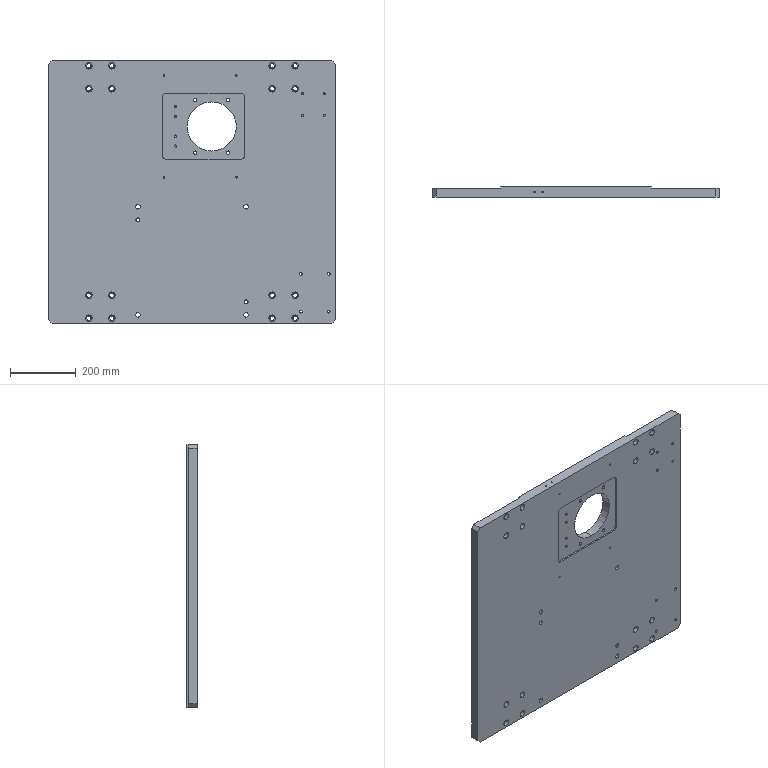Part | STEP file | HXGR200008-05-05 | 1 solid | 205 faces | box 874 x 32 x 800 mm | volume 19833550 mm3 | cylinder 134 | cone 36 | plane 35 | commonest cylinder face diameters 20 x36 13.5 x32 5 x12 6.8 x12 4.2 x8 8.5 x8